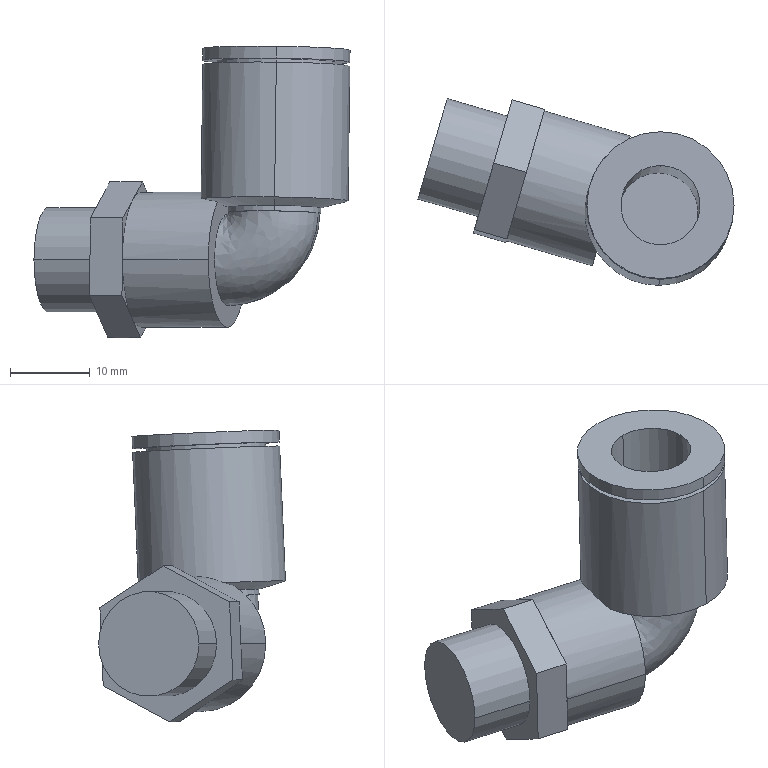Part | SolidWorks | features BaseBody 1 | 1 solid | 38 faces | box 39.742 x 23.493 x 36.691 mm | volume 9283 mm3 | plane 20 | cylinder 14 | cone 2 | spline 2 | commonest cylinder face diameters 18.5 x4 10 x2 11.729 x2 13.157 x2 15 x2 17 x2
STEP:
#1=CARTESIAN_POINT('',(-71.686,422.179,-0.7991));
#2=VERTEX_POINT('',#1);
#3=CARTESIAN_POINT('',(-71.686,403.696,-0.007463));
#4=VERTEX_POINT('',#3);
#5=CARTESIAN_POINT('',(-71.686,412.938,-0.4033));
#6=DIRECTION('',(-0.01248,-0.04279,-0.999));
#7=DIRECTION('',(0.,0.9991,-0.04279));
#8=AXIS2_PLACEMENT_3D('',#5,#6,#7);
#9=CIRCLE('',#8,9.25);
#10=EDGE_CURVE('',#2,#4,#9,.T.);
#11=ORIENTED_EDGE('',*,*,#10,.T.);
#12=CARTESIAN_POINT('',(-71.898,402.97,-16.958));
#13=VERTEX_POINT('',#12);
#14=CARTESIAN_POINT('',(-71.792,403.333,-8.483));
#15=DIRECTION('',(-0.01248,-0.04279,-0.999));
#16=VECTOR('',#15,1000.);
#17=LINE('',#14,#16);
#18=EDGE_CURVE('',#4,#13,#17,.T.);
#19=ORIENTED_EDGE('',*,*,#18,.T.);
#20=CARTESIAN_POINT('',(-71.898,421.453,-17.75));
#21=VERTEX_POINT('',#20);
#22=CARTESIAN_POINT('',(-71.898,412.212,-17.354));
#23=DIRECTION('',(0.01248,0.04279,0.999));
#24=DIRECTION('',(0.,0.9991,-0.04279));
#25=AXIS2_PLACEMENT_3D('',#22,#23,#24);
#26=CIRCLE('',#25,9.25);
#27=EDGE_CURVE('',#13,#21,#26,.T.);
#28=ORIENTED_EDGE('',*,*,#27,.T.);
#29=CARTESIAN_POINT('',(-71.792,421.816,-9.275));
#30=DIRECTION('',(-0.01248,-0.04279,-0.999));
#31=VECTOR('',#30,1000.);
#32=LINE('',#29,#31);
#33=EDGE_CURVE('',#2,#21,#32,.T.);
#34=ORIENTED_EDGE('',*,*,#33,.F.);
#35=EDGE_LOOP('',(#11,#19,#28,#34));
#36=FACE_OUTER_BOUND('',#35,.T.);
#37=CARTESIAN_POINT('',(-71.792,412.575,-8.879));
#38=DIRECTION('',(-0.01248,-0.04279,-0.999));
#39=DIRECTION('',(0.,0.9991,-0.04279));
#40=AXIS2_PLACEMENT_3D('',#37,#38,#39);
#41=CYLINDRICAL_SURFACE('',#40,9.25);
#42=ADVANCED_FACE('',(#36),#41,.T.);
#43=CARTESIAN_POINT('',(-71.909,406.314,-18.01));
#44=VERTEX_POINT('',#43);
#45=CARTESIAN_POINT('',(-71.909,418.032,-18.511));
#46=VERTEX_POINT('',#45);
#47=CARTESIAN_POINT('',(-71.909,412.173,-18.26));
#48=DIRECTION('',(0.01248,0.04279,0.999));
#49=DIRECTION('',(0.2797,0.9591,-0.04457));
#50=AXIS2_PLACEMENT_3D('',#47,#48,#49);
#51=CIRCLE('',#50,5.864);
#52=EDGE_CURVE('',#44,#46,#51,.T.);
#53=ORIENTED_EDGE('',*,*,#52,.T.);
#54=CARTESIAN_POINT('',(-71.898,421.453,-17.75));
#55=DIRECTION('',(0.003229,0.9761,0.2172));
#56=VECTOR('',#55,1000.);
#57=LINE('',#54,#56);
#58=EDGE_CURVE('',#46,#21,#57,.T.);
#59=ORIENTED_EDGE('',*,*,#58,.T.);
#60=ORIENTED_EDGE('',*,*,#27,.F.);
#61=CARTESIAN_POINT('',(-71.898,402.97,-16.958));
#62=DIRECTION('',(0.003229,-0.954,0.2999));
#63=VECTOR('',#62,1000.);
#64=LINE('',#61,#63);
#65=EDGE_CURVE('',#44,#13,#64,.T.);
#66=ORIENTED_EDGE('',*,*,#65,.F.);
#67=EDGE_LOOP('',(#53,#59,#60,#66));
#68=FACE_OUTER_BOUND('',#67,.T.);
#69=CARTESIAN_POINT('',(-71.898,412.212,-17.354));
#70=DIRECTION('',(0.01248,0.04279,0.999));
#71=DIRECTION('',(0.,-0.9991,0.04279));
#72=AXIS2_PLACEMENT_3D('',#69,#70,#71);
#73=CONICAL_SURFACE('',#72,9.25,1.309);
#74=ADVANCED_FACE('',(#68),#73,.T.);
#75=CARTESIAN_POINT('',(-91.031,408.596,-24.5));
#76=VERTEX_POINT('',#75);
#77=CARTESIAN_POINT('',(-91.033,408.588,-24.879));
#78=VERTEX_POINT('',#77);
#79=CARTESIAN_POINT('',(-88.653,416.748,-24.879));
#80=DIRECTION('',(0.96,-0.28,0.));
#81=DIRECTION('',(0.28,0.96,0.));
#82=AXIS2_PLACEMENT_3D('',#79,#80,#81);
#83=CIRCLE('',#82,8.5);
#84=EDGE_CURVE('',#76,#78,#83,.T.);
#85=ORIENTED_EDGE('',*,*,#84,.T.);
#86=CARTESIAN_POINT('',(-80.232,405.438,-24.879));
#87=VERTEX_POINT('',#86);
#88=CARTESIAN_POINT('',(-87.546,407.571,-24.879));
#89=DIRECTION('',(0.96,-0.28,0.));
#90=VECTOR('',#89,1000.);
#91=LINE('',#88,#90);
#92=EDGE_CURVE('',#78,#87,#91,.T.);
#93=ORIENTED_EDGE('',*,*,#92,.T.);
#94=CARTESIAN_POINT('',(-79.066,409.437,-17.567));
#95=VERTEX_POINT('',#94);
#96=CARTESIAN_POINT('',(-77.852,413.598,-24.879));
#97=DIRECTION('',(-0.96,0.28,0.));
#98=DIRECTION('',(0.28,0.96,0.));
#99=AXIS2_PLACEMENT_3D('',#96,#97,#98);
#100=CIRCLE('',#99,8.5);
#101=EDGE_CURVE('',#87,#95,#100,.T.);
#102=ORIENTED_EDGE('',*,*,#101,.T.);
#103=CARTESIAN_POINT('',(-81.034,410.777,-17.179));
#104=VERTEX_POINT('',#103);
#105=CARTESIAN_POINT('',(-81.034,410.777,-17.179));
#106=CARTESIAN_POINT('',(-80.404,410.293,-17.313));
#107=CARTESIAN_POINT('',(-79.746,409.85,-17.445));
#108=CARTESIAN_POINT('',(-79.066,409.437,-17.567));
#109=B_SPLINE_CURVE_WITH_KNOTS('',3,(#105,#106,#107,#108),.UNSPECIFIED.,.F.,.F.,(4,4),(0.,0.002412),.UNSPECIFIED.);
#110=EDGE_CURVE('',#104,#95,#109,.T.);
#111=ORIENTED_EDGE('',*,*,#110,.F.);
#112=CARTESIAN_POINT('',(-78.831,418.333,-17.53));
#113=VERTEX_POINT('',#112);
#114=CARTESIAN_POINT('',(-78.831,418.333,-17.53));
#115=CARTESIAN_POINT('',(-79.25,417.867,-17.202));
#116=CARTESIAN_POINT('',(-79.631,417.344,-16.934));
#117=CARTESIAN_POINT('',(-80.129,416.459,-16.637));
#118=CARTESIAN_POINT('',(-80.281,416.148,-16.558));
#119=CARTESIAN_POINT('',(-80.55,415.511,-16.441));
#120=CARTESIAN_POINT('',(-80.667,415.182,-16.403));
#121=CARTESIAN_POINT('',(-80.964,414.161,-16.356));
#122=CARTESIAN_POINT('',(-81.08,413.476,-16.413));
#123=CARTESIAN_POINT('',(-81.143,412.44,-16.618));
#124=CARTESIAN_POINT('',(-81.145,412.097,-16.707));
#125=CARTESIAN_POINT('',(-81.114,411.427,-16.918));
#126=CARTESIAN_POINT('',(-81.082,411.099,-17.04));
#127=CARTESIAN_POINT('',(-81.034,410.777,-17.179));
#128=B_SPLINE_CURVE_WITH_KNOTS('',3,(#114,#115,#116,#117,#118,#119,#120,#121,#122,#123,#124,#125,#126,#127),.UNSPECIFIED.,.F.,.F.,(4,2,2,2,2,2,4),(-0.004184,-0.002092,-0.001045,0.000001124,0.002094,0.00314,0.004187),.UNSPECIFIED.);
#129=EDGE_CURVE('',#113,#104,#128,.T.);
#130=ORIENTED_EDGE('',*,*,#129,.F.);
#131=CARTESIAN_POINT('',(-76.461,418.369,-17.983));
#132=VERTEX_POINT('',#131);
#133=CARTESIAN_POINT('',(-78.831,418.333,-17.53));
#134=CARTESIAN_POINT('',(-78.043,418.389,-17.69));
#135=CARTESIAN_POINT('',(-77.254,418.397,-17.843));
#136=CARTESIAN_POINT('',(-76.461,418.369,-17.983));
#137=B_SPLINE_CURVE_WITH_KNOTS('',3,(#133,#134,#135,#136),.UNSPECIFIED.,.F.,.F.,(4,4),(0.,0.002412),.UNSPECIFIED.);
#138=EDGE_CURVE('',#113,#132,#137,.T.);
#139=ORIENTED_EDGE('',*,*,#138,.T.);
#140=CARTESIAN_POINT('',(-75.473,421.759,-24.879));
#141=VERTEX_POINT('',#140);
#142=CARTESIAN_POINT('',(-77.852,413.598,-24.879));
#143=DIRECTION('',(-0.96,0.28,0.));
#144=DIRECTION('',(0.28,0.96,0.));
#145=AXIS2_PLACEMENT_3D('',#142,#143,#144);
#146=CIRCLE('',#145,8.5);
#147=EDGE_CURVE('',#132,#141,#146,.T.);
#148=ORIENTED_EDGE('',*,*,#147,.T.);
#149=CARTESIAN_POINT('',(-86.274,424.908,-24.879));
#150=VERTEX_POINT('',#149);
#151=CARTESIAN_POINT('',(-82.787,423.892,-24.879));
#152=DIRECTION('',(0.96,-0.28,0.));
#153=VECTOR('',#152,1000.);
#154=LINE('',#151,#153);
#155=EDGE_CURVE('',#150,#141,#154,.T.);
#156=ORIENTED_EDGE('',*,*,#155,.F.);
#157=CARTESIAN_POINT('',(-87.373,421.139,-17.714));
#158=VERTEX_POINT('',#157);
#159=CARTESIAN_POINT('',(-88.653,416.748,-24.879));
#160=DIRECTION('',(0.96,-0.28,0.));
#161=DIRECTION('',(0.28,0.96,0.));
#162=AXIS2_PLACEMENT_3D('',#159,#160,#161);
#163=CIRCLE('',#162,8.5);
#164=EDGE_CURVE('',#150,#158,#163,.T.);
#165=ORIENTED_EDGE('',*,*,#164,.T.);
#166=CARTESIAN_POINT('',(-89.75,412.987,-17.336));
#167=VERTEX_POINT('',#166);
#168=CARTESIAN_POINT('',(-88.653,416.748,-24.879));
#169=DIRECTION('',(0.96,-0.28,0.));
#170=DIRECTION('',(0.28,0.96,0.));
#171=AXIS2_PLACEMENT_3D('',#168,#169,#170);
#172=CIRCLE('',#171,8.5);
#173=EDGE_CURVE('',#158,#167,#172,.T.);
#174=ORIENTED_EDGE('',*,*,#173,.T.);
#175=CARTESIAN_POINT('',(-88.653,416.748,-24.879));
#176=DIRECTION('',(0.96,-0.28,0.));
#177=DIRECTION('',(0.28,0.96,0.));
#178=AXIS2_PLACEMENT_3D('',#175,#176,#177);
#179=CIRCLE('',#178,8.5);
#180=EDGE_CURVE('',#167,#76,#179,.T.);
#181=ORIENTED_EDGE('',*,*,#180,.T.);
#182=EDGE_LOOP('',(#85,#93,#102,#111,#130,#139,#148,#156,#165,#174,#181));
#183=FACE_OUTER_BOUND('',#182,.T.);
#184=CARTESIAN_POINT('',(-85.167,415.731,-24.879));
#185=DIRECTION('',(0.96,-0.28,0.));
#186=DIRECTION('',(0.28,0.96,0.));
#187=AXIS2_PLACEMENT_3D('',#184,#185,#186);
#188=CYLINDRICAL_SURFACE('',#187,8.5);
#189=ADVANCED_FACE('',(#183),#188,.T.);
#190=CARTESIAN_POINT('',(-71.68,420.452,-0.2247));
#191=VERTEX_POINT('',#190);
#192=CARTESIAN_POINT('',(-71.68,405.466,0.4172));
#193=VERTEX_POINT('',#192);
#194=CARTESIAN_POINT('',(-71.68,412.959,0.09624));
#195=DIRECTION('',(-0.01248,-0.04279,-0.999));
#196=DIRECTION('',(0.,0.9991,-0.04279));
#197=AXIS2_PLACEMENT_3D('',#194,#195,#196);
#198=CIRCLE('',#197,7.5);
#199=EDGE_CURVE('',#191,#193,#198,.T.);
#200=ORIENTED_EDGE('',*,*,#199,.T.);
#201=CARTESIAN_POINT('',(-71.686,405.444,-0.08234));
#202=VERTEX_POINT('',#201);
#203=CARTESIAN_POINT('',(-71.683,405.455,0.1674));
#204=DIRECTION('',(-0.01248,-0.04279,-0.999));
#205=VECTOR('',#204,1000.);
#206=LINE('',#203,#205);
#207=EDGE_CURVE('',#193,#202,#206,.T.);
#208=ORIENTED_EDGE('',*,*,#207,.T.);
#209=CARTESIAN_POINT('',(-71.686,420.431,-0.7242));
#210=VERTEX_POINT('',#209);
#211=CARTESIAN_POINT('',(-71.686,412.938,-0.4033));
#212=DIRECTION('',(-0.01248,-0.04279,-0.999));
#213=DIRECTION('',(0.,0.9991,-0.04279));
#214=AXIS2_PLACEMENT_3D('',#211,#212,#213);
#215=CIRCLE('',#214,7.5);
#216=EDGE_CURVE('',#210,#202,#215,.T.);
#217=ORIENTED_EDGE('',*,*,#216,.F.);
#218=CARTESIAN_POINT('',(-71.683,420.441,-0.4744));
#219=DIRECTION('',(-0.01248,-0.04279,-0.999));
#220=VECTOR('',#219,1000.);
#221=LINE('',#218,#220);
#222=EDGE_CURVE('',#191,#210,#221,.T.);
#223=ORIENTED_EDGE('',*,*,#222,.F.);
#224=EDGE_LOOP('',(#200,#208,#217,#223));
#225=FACE_OUTER_BOUND('',#224,.T.);
#226=CARTESIAN_POINT('',(-71.683,412.948,-0.1535));
#227=DIRECTION('',(-0.01248,-0.04279,-0.999));
#228=DIRECTION('',(0.,0.9991,-0.04279));
#229=AXIS2_PLACEMENT_3D('',#226,#227,#228);
#230=CYLINDRICAL_SURFACE('',#229,7.5);
#231=ADVANCED_FACE('',(#225),#230,.T.);
#232=ORIENTED_EDGE('',*,*,#52,.F.);
#233=CARTESIAN_POINT('',(-71.918,406.284,-18.714));
#234=VERTEX_POINT('',#233);
#235=CARTESIAN_POINT('',(-71.913,406.299,-18.362));
#236=DIRECTION('',(-0.01248,-0.04279,-0.999));
#237=VECTOR('',#236,1000.);
#238=LINE('',#235,#237);
#239=EDGE_CURVE('',#44,#234,#238,.T.);
#240=ORIENTED_EDGE('',*,*,#239,.T.);
#241=CARTESIAN_POINT('',(-71.918,418.002,-19.216));
#242=VERTEX_POINT('',#241);
#243=CARTESIAN_POINT('',(-71.918,412.143,-18.965));
#244=DIRECTION('',(0.01248,0.04279,0.999));
#245=DIRECTION('',(0.,0.9991,-0.04279));
#246=AXIS2_PLACEMENT_3D('',#243,#244,#245);
#247=CIRCLE('',#246,5.864);
#248=EDGE_CURVE('',#234,#242,#247,.T.);
#249=ORIENTED_EDGE('',*,*,#248,.T.);
#250=CARTESIAN_POINT('',(-71.913,418.017,-18.864));
#251=DIRECTION('',(-0.01248,-0.04279,-0.999));
#252=VECTOR('',#251,1000.);
#253=LINE('',#250,#252);
#254=EDGE_CURVE('',#46,#242,#253,.T.);
#255=ORIENTED_EDGE('',*,*,#254,.F.);
#256=EDGE_LOOP('',(#232,#240,#249,#255));
#257=FACE_OUTER_BOUND('',#256,.T.);
#258=CARTESIAN_POINT('',(-71.913,412.158,-18.613));
#259=DIRECTION('',(-0.01248,-0.04279,-0.999));
#260=DIRECTION('',(0.,0.9991,-0.04279));
#261=AXIS2_PLACEMENT_3D('',#258,#259,#260);
#262=CYLINDRICAL_SURFACE('',#261,5.864);
#263=ADVANCED_FACE('',(#257),#262,.T.);
#264=CARTESIAN_POINT('',(-71.661,422.265,1.199));
#265=VERTEX_POINT('',#264);
#266=CARTESIAN_POINT('',(-71.661,403.782,1.991));
#267=VERTEX_POINT('',#266);
#268=CARTESIAN_POINT('',(-71.661,413.023,1.595));
#269=DIRECTION('',(-0.01248,-0.04279,-0.999));
#270=DIRECTION('',(0.,0.9991,-0.04279));
#271=AXIS2_PLACEMENT_3D('',#268,#269,#270);
#272=CIRCLE('',#271,9.25);
#273=EDGE_CURVE('',#265,#267,#272,.T.);
#274=ORIENTED_EDGE('',*,*,#273,.T.);
#275=CARTESIAN_POINT('',(-71.68,403.717,0.492));
#276=VERTEX_POINT('',#275);
#277=CARTESIAN_POINT('',(-71.67,403.75,1.241));
#278=DIRECTION('',(-0.01248,-0.04279,-0.999));
#279=VECTOR('',#278,1000.);
#280=LINE('',#277,#279);
#281=EDGE_CURVE('',#267,#276,#280,.T.);
#282=ORIENTED_EDGE('',*,*,#281,.T.);
#283=CARTESIAN_POINT('',(-71.68,422.201,-0.2996));
#284=VERTEX_POINT('',#283);
#285=CARTESIAN_POINT('',(-71.68,412.959,0.09624));
#286=DIRECTION('',(-0.01248,-0.04279,-0.999));
#287=DIRECTION('',(0.,0.9991,-0.04279));
#288=AXIS2_PLACEMENT_3D('',#285,#286,#287);
#289=CIRCLE('',#288,9.25);
#290=EDGE_CURVE('',#284,#276,#289,.T.);
#291=ORIENTED_EDGE('',*,*,#290,.F.);
#292=CARTESIAN_POINT('',(-71.67,422.233,0.4497));
#293=DIRECTION('',(-0.01248,-0.04279,-0.999));
#294=VECTOR('',#293,1000.);
#295=LINE('',#292,#294);
#296=EDGE_CURVE('',#265,#284,#295,.T.);
#297=ORIENTED_EDGE('',*,*,#296,.F.);
#298=EDGE_LOOP('',(#274,#282,#291,#297));
#299=FACE_OUTER_BOUND('',#298,.T.);
#300=CARTESIAN_POINT('',(-71.67,412.991,0.8455));
#301=DIRECTION('',(-0.01248,-0.04279,-0.999));
#302=DIRECTION('',(0.,0.9991,-0.04279));
#303=AXIS2_PLACEMENT_3D('',#300,#301,#302);
#304=CYLINDRICAL_SURFACE('',#303,9.25);
#305=ADVANCED_FACE('',(#299),#304,.T.);
#306=CARTESIAN_POINT('',(-98.47,426.463,-24.879));
#307=VERTEX_POINT('',#306);
#308=CARTESIAN_POINT('',(-102.154,413.833,-24.879));
#309=VERTEX_POINT('',#308);
#310=CARTESIAN_POINT('',(-100.312,420.148,-24.879));
#311=DIRECTION('',(0.96,-0.28,0.));
#312=DIRECTION('',(0.28,0.96,0.));
#313=AXIS2_PLACEMENT_3D('',#310,#311,#312);
#314=CIRCLE('',#313,6.579);
#315=EDGE_CURVE('',#307,#309,#314,.T.);
#316=ORIENTED_EDGE('',*,*,#315,.T.);
#317=CARTESIAN_POINT('',(-94.575,411.623,-24.879));
#318=VERTEX_POINT('',#317);
#319=CARTESIAN_POINT('',(-98.238,412.691,-24.879));
#320=DIRECTION('',(0.96,-0.28,0.));
#321=VECTOR('',#320,1000.);
#322=LINE('',#319,#321);
#323=EDGE_CURVE('',#309,#318,#322,.T.);
#324=ORIENTED_EDGE('',*,*,#323,.T.);
#325=CARTESIAN_POINT('',(-90.892,424.253,-24.879));
#326=VERTEX_POINT('',#325);
#327=CARTESIAN_POINT('',(-92.733,417.938,-24.879));
#328=DIRECTION('',(-0.96,0.28,0.));
#329=DIRECTION('',(0.28,0.96,0.));
#330=AXIS2_PLACEMENT_3D('',#327,#328,#329);
#331=CIRCLE('',#330,6.579);
#332=EDGE_CURVE('',#318,#326,#331,.T.);
#333=ORIENTED_EDGE('',*,*,#332,.T.);
#334=CARTESIAN_POINT('',(-94.555,425.322,-24.879));
#335=DIRECTION('',(0.96,-0.28,0.));
#336=VECTOR('',#335,1000.);
#337=LINE('',#334,#336);
#338=EDGE_CURVE('',#307,#326,#337,.T.);
#339=ORIENTED_EDGE('',*,*,#338,.F.);
#340=EDGE_LOOP('',(#316,#324,#333,#339));
#341=FACE_OUTER_BOUND('',#340,.T.);
#342=CARTESIAN_POINT('',(-96.396,419.006,-24.879));
#343=DIRECTION('',(0.96,-0.28,0.));
#344=DIRECTION('',(0.28,0.96,0.));
#345=AXIS2_PLACEMENT_3D('',#342,#343,#344);
#346=CYLINDRICAL_SURFACE('',#345,6.579);
#347=ADVANCED_FACE('',(#341),#346,.T.);
#348=CARTESIAN_POINT('',(-71.923,417.12,-19.598));
#349=VERTEX_POINT('',#348);
#350=CARTESIAN_POINT('',(-71.923,407.129,-19.17));
#351=VERTEX_POINT('',#350);
#352=CARTESIAN_POINT('',(-71.923,412.125,-19.384));
#353=DIRECTION('',(0.01248,0.04279,0.999));
#354=DIRECTION('',(0.,-0.9991,0.04279));
#355=AXIS2_PLACEMENT_3D('',#352,#353,#354);
#356=CIRCLE('',#355,5.);
#357=EDGE_CURVE('',#349,#351,#356,.T.);
#358=ORIENTED_EDGE('',*,*,#357,.F.);
#359=CARTESIAN_POINT('',(-71.661,418.019,1.381));
#360=VERTEX_POINT('',#359);
#361=CARTESIAN_POINT('',(-71.399,418.917,22.36));
#362=DIRECTION('',(0.01248,0.04279,0.999));
#363=VECTOR('',#362,1000.);
#364=LINE('',#361,#363);
#365=EDGE_CURVE('',#349,#360,#364,.T.);
#366=ORIENTED_EDGE('',*,*,#365,.T.);
#367=CARTESIAN_POINT('',(-71.661,408.028,1.809));
#368=VERTEX_POINT('',#367);
#369=CARTESIAN_POINT('',(-71.661,413.023,1.595));
#370=DIRECTION('',(-0.01248,-0.04279,-0.999));
#371=DIRECTION('',(0.,-0.9991,0.04279));
#372=AXIS2_PLACEMENT_3D('',#369,#370,#371);
#373=CIRCLE('',#372,5.);
#374=EDGE_CURVE('',#368,#360,#373,.T.);
#375=ORIENTED_EDGE('',*,*,#374,.F.);
#376=CARTESIAN_POINT('',(-71.399,408.926,22.788));
#377=DIRECTION('',(0.01248,0.04279,0.999));
#378=VECTOR('',#377,1000.);
#379=LINE('',#376,#378);
#380=EDGE_CURVE('',#351,#368,#379,.T.);
#381=ORIENTED_EDGE('',*,*,#380,.F.);
#382=EDGE_LOOP('',(#358,#366,#375,#381));
#383=FACE_OUTER_BOUND('',#382,.T.);
#384=CARTESIAN_POINT('',(-71.399,413.922,22.574));
#385=DIRECTION('',(0.01248,0.04279,0.999));
#386=DIRECTION('',(0.,-0.9991,0.04279));
#387=AXIS2_PLACEMENT_3D('',#384,#385,#386);
#388=CYLINDRICAL_SURFACE('',#387,5.);
#389=ADVANCED_FACE('',(#383),#388,.F.);
#390=ORIENTED_EDGE('',*,*,#18,.F.);
#391=CARTESIAN_POINT('',(-71.686,412.938,-0.4033));
#392=DIRECTION('',(-0.01248,-0.04279,-0.999));
#393=DIRECTION('',(0.,0.9991,-0.04279));
#394=AXIS2_PLACEMENT_3D('',#391,#392,#393);
#395=CIRCLE('',#394,9.25);
#396=EDGE_CURVE('',#4,#2,#395,.T.);
#397=ORIENTED_EDGE('',*,*,#396,.T.);
#398=ORIENTED_EDGE('',*,*,#33,.T.);
#399=CARTESIAN_POINT('',(-71.898,412.212,-17.354));
#400=DIRECTION('',(0.01248,0.04279,0.999));
#401=DIRECTION('',(0.,0.9991,-0.04279));
#402=AXIS2_PLACEMENT_3D('',#399,#400,#401);
#403=CIRCLE('',#402,9.25);
#404=EDGE_CURVE('',#21,#113,#403,.T.);
#405=ORIENTED_EDGE('',*,*,#404,.T.);
#406=ORIENTED_EDGE('',*,*,#129,.T.);
#407=CARTESIAN_POINT('',(-71.898,412.212,-17.354));
#408=DIRECTION('',(0.01248,0.04279,0.999));
#409=DIRECTION('',(0.,0.9991,-0.04279));
#410=AXIS2_PLACEMENT_3D('',#407,#408,#409);
#411=CIRCLE('',#410,9.25);
#412=EDGE_CURVE('',#104,#13,#411,.T.);
#413=ORIENTED_EDGE('',*,*,#412,.T.);
#414=EDGE_LOOP('',(#390,#397,#398,#405,#406,#413));
#415=FACE_OUTER_BOUND('',#414,.T.);
#416=CARTESIAN_POINT('',(-71.792,412.575,-8.879));
#417=DIRECTION('',(-0.01248,-0.04279,-0.999));
#418=DIRECTION('',(0.,0.9991,-0.04279));
#419=AXIS2_PLACEMENT_3D('',#416,#417,#418);
#420=CYLINDRICAL_SURFACE('',#419,9.25);
#421=ADVANCED_FACE('',(#415),#420,.T.);
#422=ORIENTED_EDGE('',*,*,#216,.T.);
#423=CARTESIAN_POINT('',(-71.686,412.938,-0.4033));
#424=DIRECTION('',(-0.01248,-0.04279,-0.999));
#425=DIRECTION('',(0.,0.9991,-0.04279));
#426=AXIS2_PLACEMENT_3D('',#423,#424,#425);
#427=CIRCLE('',#426,7.5);
#428=EDGE_CURVE('',#202,#210,#427,.T.);
#429=ORIENTED_EDGE('',*,*,#428,.T.);
#430=EDGE_LOOP('',(#422,#429));
#431=FACE_BOUND('',#430,.T.);
#432=ORIENTED_EDGE('',*,*,#10,.F.);
#433=ORIENTED_EDGE('',*,*,#396,.F.);
#434=EDGE_LOOP('',(#432,#433));
#435=FACE_OUTER_BOUND('',#434,.T.);
#436=CARTESIAN_POINT('',(-69.344,420.97,-0.7765));
#437=DIRECTION('',(0.01248,0.04279,0.999));
#438=DIRECTION('',(0.,-0.9991,0.04279));
#439=AXIS2_PLACEMENT_3D('',#436,#437,#438);
#440=PLANE('',#439);
#441=ADVANCED_FACE('',(#431,#435),#440,.T.);
#442=ORIENTED_EDGE('',*,*,#58,.F.);
#443=CARTESIAN_POINT('',(-71.909,412.173,-18.26));
#444=DIRECTION('',(0.01248,0.04279,0.999));
#445=DIRECTION('',(0.2797,0.9591,-0.04457));
#446=AXIS2_PLACEMENT_3D('',#443,#444,#445);
#447=CIRCLE('',#446,5.864);
#448=EDGE_CURVE('',#46,#44,#447,.T.);
#449=ORIENTED_EDGE('',*,*,#448,.T.);
#450=ORIENTED_EDGE('',*,*,#65,.T.);
#451=ORIENTED_EDGE('',*,*,#412,.F.);
#452=ORIENTED_EDGE('',*,*,#110,.T.);
#453=CARTESIAN_POINT('',(-79.066,409.437,-17.567));
#454=CARTESIAN_POINT('',(-78.852,410.171,-17.727));
#455=CARTESIAN_POINT('',(-78.637,410.908,-17.868));
#456=CARTESIAN_POINT('',(-78.205,412.389,-18.085));
#457=CARTESIAN_POINT('',(-77.988,413.134,-18.161));
#458=CARTESIAN_POINT('',(-77.55,414.635,-18.231));
#459=CARTESIAN_POINT('',(-77.332,415.384,-18.224));
#460=CARTESIAN_POINT('',(-76.896,416.878,-18.145));
#461=CARTESIAN_POINT('',(-76.679,417.624,-18.073));
#462=CARTESIAN_POINT('',(-76.461,418.369,-17.983));
#463=B_SPLINE_CURVE_WITH_KNOTS('',3,(#453,#454,#455,#456,#457,#458,#459,#460,#461,#462),.UNSPECIFIED.,.F.,.F.,(4,2,2,2,4),(0.,0.002338,0.004676,0.007013,0.009351),.UNSPECIFIED.);
#464=EDGE_CURVE('',#95,#132,#463,.T.);
#465=ORIENTED_EDGE('',*,*,#464,.T.);
#466=ORIENTED_EDGE('',*,*,#138,.F.);
#467=ORIENTED_EDGE('',*,*,#404,.F.);
#468=EDGE_LOOP('',(#442,#449,#450,#451,#452,#465,#466,#467));
#469=FACE_OUTER_BOUND('',#468,.T.);
#470=CARTESIAN_POINT('',(-71.898,412.212,-17.354));
#471=DIRECTION('',(0.01248,0.04279,0.999));
#472=DIRECTION('',(0.,-0.9991,0.04279));
#473=AXIS2_PLACEMENT_3D('',#470,#471,#472);
#474=CONICAL_SURFACE('',#473,9.25,1.309);
#475=ADVANCED_FACE('',(#469),#474,.T.);
#476=ORIENTED_EDGE('',*,*,#92,.F.);
#477=CARTESIAN_POINT('',(-89.934,412.357,-32.043));
#478=VERTEX_POINT('',#477);
#479=CARTESIAN_POINT('',(-88.653,416.748,-24.879));
#480=DIRECTION('',(0.96,-0.28,0.));
#481=DIRECTION('',(0.28,0.96,0.));
#482=AXIS2_PLACEMENT_3D('',#479,#480,#481);
#483=CIRCLE('',#482,8.5);
#484=EDGE_CURVE('',#78,#478,#483,.T.);
#485=ORIENTED_EDGE('',*,*,#484,.T.);
#486=CARTESIAN_POINT('',(-87.557,420.509,-32.422));
#487=VERTEX_POINT('',#486);
#488=CARTESIAN_POINT('',(-88.653,416.748,-24.879));
#489=DIRECTION('',(0.96,-0.28,0.));
#490=DIRECTION('',(0.28,0.96,0.));
#491=AXIS2_PLACEMENT_3D('',#488,#489,#490);
#492=CIRCLE('',#491,8.5);
#493=EDGE_CURVE('',#478,#487,#492,.T.);
#494=ORIENTED_EDGE('',*,*,#493,.T.);
#495=CARTESIAN_POINT('',(-86.276,424.9,-25.258));
#496=VERTEX_POINT('',#495);
#497=CARTESIAN_POINT('',(-88.653,416.748,-24.879));
#498=DIRECTION('',(0.96,-0.28,0.));
#499=DIRECTION('',(0.28,0.96,0.));
#500=AXIS2_PLACEMENT_3D('',#497,#498,#499);
#501=CIRCLE('',#500,8.5);
#502=EDGE_CURVE('',#487,#496,#501,.T.);
#503=ORIENTED_EDGE('',*,*,#502,.T.);
#504=CARTESIAN_POINT('',(-88.653,416.748,-24.879));
#505=DIRECTION('',(0.96,-0.28,0.));
#506=DIRECTION('',(0.28,0.96,0.));
#507=AXIS2_PLACEMENT_3D('',#504,#505,#506);
#508=CIRCLE('',#507,8.5);
#509=EDGE_CURVE('',#496,#150,#508,.T.);
#510=ORIENTED_EDGE('',*,*,#509,.T.);
#511=ORIENTED_EDGE('',*,*,#155,.T.);
#512=CARTESIAN_POINT('',(-77.852,413.598,-24.879));
#513=DIRECTION('',(-0.96,0.28,0.));
#514=DIRECTION('',(0.28,0.96,0.));
#515=AXIS2_PLACEMENT_3D('',#512,#513,#514);
#516=CIRCLE('',#515,8.5);
#517=EDGE_CURVE('',#141,#87,#516,.T.);
#518=ORIENTED_EDGE('',*,*,#517,.T.);
#519=EDGE_LOOP('',(#476,#485,#494,#503,#510,#511,#518));
#520=FACE_OUTER_BOUND('',#519,.T.);
#521=CARTESIAN_POINT('',(-85.167,415.731,-24.879));
#522=DIRECTION('',(0.96,-0.28,0.));
#523=DIRECTION('',(0.28,0.96,0.));
#524=AXIS2_PLACEMENT_3D('',#521,#522,#523);
#525=CYLINDRICAL_SURFACE('',#524,8.5);
#526=ADVANCED_FACE('',(#520),#525,.T.);
#527=ORIENTED_EDGE('',*,*,#207,.F.);
#528=CARTESIAN_POINT('',(-71.68,412.959,0.09624));
#529=DIRECTION('',(-0.01248,-0.04279,-0.999));
#530=DIRECTION('',(0.,0.9991,-0.04279));
#531=AXIS2_PLACEMENT_3D('',#528,#529,#530);
#532=CIRCLE('',#531,7.5);
#533=EDGE_CURVE('',#193,#191,#532,.T.);
#534=ORIENTED_EDGE('',*,*,#533,.T.);
#535=ORIENTED_EDGE('',*,*,#222,.T.);
#536=ORIENTED_EDGE('',*,*,#428,.F.);
#537=EDGE_LOOP('',(#527,#534,#535,#536));
#538=FACE_OUTER_BOUND('',#537,.T.);
#539=CARTESIAN_POINT('',(-71.683,412.948,-0.1535));
#540=DIRECTION('',(-0.01248,-0.04279,-0.999));
#541=DIRECTION('',(0.,0.9991,-0.04279));
#542=AXIS2_PLACEMENT_3D('',#539,#540,#541);
#543=CYLINDRICAL_SURFACE('',#542,7.5);
#544=ADVANCED_FACE('',(#538),#543,.T.);
#545=ORIENTED_EDGE('',*,*,#464,.F.);
#546=ORIENTED_EDGE('',*,*,#101,.F.);
#547=ORIENTED_EDGE('',*,*,#517,.F.);
#548=ORIENTED_EDGE('',*,*,#147,.F.);
#549=EDGE_LOOP('',(#545,#546,#547,#548));
#550=FACE_OUTER_BOUND('',#549,.T.);
#551=CARTESIAN_POINT('',(-77.924,413.353,-30.608));
#552=VERTEX_POINT('',#551);
#553=CARTESIAN_POINT('',(-77.781,413.844,-19.15));
#554=VERTEX_POINT('',#553);
#555=CARTESIAN_POINT('',(-77.924,413.353,-30.608));
#556=CARTESIAN_POINT('',(-78.03,412.99,-30.591));
#557=CARTESIAN_POINT('',(-78.134,412.634,-30.538));
#558=CARTESIAN_POINT('',(-78.286,412.112,-30.404));
#559=CARTESIAN_POINT('',(-78.336,411.939,-30.351));
#560=CARTESIAN_POINT('',(-78.436,411.598,-30.225));
#561=CARTESIAN_POINT('',(-78.485,411.429,-30.153));
#562=CARTESIAN_POINT('',(-78.628,410.939,-29.915));
#563=CARTESIAN_POINT('',(-78.718,410.631,-29.724));
#564=CARTESIAN_POINT('',(-78.887,410.051,-29.281));
#565=CARTESIAN_POINT('',(-78.967,409.778,-29.025));
#566=CARTESIAN_POINT('',(-79.108,409.293,-28.473));
#567=CARTESIAN_POINT('',(-79.171,409.078,-28.174));
#568=CARTESIAN_POINT('',(-79.253,408.797,-27.691));
#569=CARTESIAN_POINT('',(-79.278,408.71,-27.524));
#570=CARTESIAN_POINT('',(-79.323,408.554,-27.185));
#571=CARTESIAN_POINT('',(-79.344,408.485,-27.013));
#572=CARTESIAN_POINT('',(-79.397,408.301,-26.486));
#573=CARTESIAN_POINT('',(-79.423,408.211,-26.12));
#574=CARTESIAN_POINT('',(-79.455,408.101,-25.374));
#575=CARTESIAN_POINT('',(-79.461,408.082,-25.001));
#576=CARTESIAN_POINT('',(-79.452,408.114,-24.254));
#577=CARTESIAN_POINT('',(-79.437,408.166,-23.876));
#578=CARTESIAN_POINT('',(-79.387,408.337,-23.148));
#579=CARTESIAN_POINT('',(-79.352,408.456,-22.795));
#580=CARTESIAN_POINT('',(-79.285,408.685,-22.285));
#581=CARTESIAN_POINT('',(-79.26,408.77,-22.116));
#582=CARTESIAN_POINT('',(-79.207,408.955,-21.792));
#583=CARTESIAN_POINT('',(-79.178,409.054,-21.636));
#584=CARTESIAN_POINT('',(-79.085,409.372,-21.184));
#585=CARTESIAN_POINT('',(-79.015,409.612,-20.905));
#586=CARTESIAN_POINT('',(-78.859,410.148,-20.394));
#587=CARTESIAN_POINT('',(-78.775,410.436,-20.169));
#588=CARTESIAN_POINT('',(-78.64,410.896,-19.879));
#589=CARTESIAN_POINT('',(-78.594,411.054,-19.79));
#590=CARTESIAN_POINT('',(-78.499,411.38,-19.627));
#591=CARTESIAN_POINT('',(-78.45,411.548,-19.553));
#592=CARTESIAN_POINT('',(-78.302,412.057,-19.36));
#593=CARTESIAN_POINT('',(-78.201,412.405,-19.268));
#594=CARTESIAN_POINT('',(-77.993,413.115,-19.154));
#595=CARTESIAN_POINT('',(-77.887,413.481,-19.133));
#596=CARTESIAN_POINT('',(-77.781,413.844,-19.15));
#597=B_SPLINE_CURVE_WITH_KNOTS('',3,(#555,#556,#557,#558,#559,#560,#561,#562,#563,#564,#565,#566,#567,#568,#569,#570,#571,#572,#573,#574,#575,#576,#577,#578,#579,#580,#581,#582,#583,#584,#585,#586,#587,#588,#589,#590,#591,#592,#593,#594,#595,#596),.UNSPECIFIED.,.F.,.F.,(4,2,2,2,2,2,2,2,2,2,2,2,2,2,2,2,2,2,2,2,4),(0.,0.00112,0.001681,0.002241,0.003361,0.004482,0.005602,0.006162,0.006722,0.007843,0.008963,0.01008,0.0112,0.01176,0.01232,0.01344,0.01457,0.01513,0.01569,0.01681,0.01793),.UNSPECIFIED.);
#598=EDGE_CURVE('',#552,#554,#597,.T.);
#599=ORIENTED_EDGE('',*,*,#598,.T.);
#600=CARTESIAN_POINT('',(-77.781,413.844,-19.15));
#601=CARTESIAN_POINT('',(-77.675,414.207,-19.166));
#602=CARTESIAN_POINT('',(-77.569,414.569,-19.221));
#603=CARTESIAN_POINT('',(-77.365,415.269,-19.401));
#604=CARTESIAN_POINT('',(-77.267,415.607,-19.526));
#605=CARTESIAN_POINT('',(-77.077,416.259,-19.844));
#606=CARTESIAN_POINT('',(-76.985,416.574,-20.039));
#607=CARTESIAN_POINT('',(-76.816,417.152,-20.482));
#608=CARTESIAN_POINT('',(-76.738,417.419,-20.732));
#609=CARTESIAN_POINT('',(-76.596,417.908,-21.29));
#610=CARTESIAN_POINT('',(-76.533,418.124,-21.592));
#611=CARTESIAN_POINT('',(-76.452,418.402,-22.071));
#612=CARTESIAN_POINT('',(-76.427,418.488,-22.235));
#613=CARTESIAN_POINT('',(-76.381,418.643,-22.574));
#614=CARTESIAN_POINT('',(-76.361,418.714,-22.749));
#615=CARTESIAN_POINT('',(-76.307,418.898,-23.281));
#616=CARTESIAN_POINT('',(-76.281,418.987,-23.643));
#617=CARTESIAN_POINT('',(-76.249,419.095,-24.383));
#618=CARTESIAN_POINT('',(-76.244,419.115,-24.764));
#619=CARTESIAN_POINT('',(-76.253,419.082,-25.512));
#620=CARTESIAN_POINT('',(-76.268,419.031,-25.882));
#621=CARTESIAN_POINT('',(-76.306,418.902,-26.43));
#622=CARTESIAN_POINT('',(-76.321,418.85,-26.612));
#623=CARTESIAN_POINT('',(-76.356,418.73,-26.966));
#624=CARTESIAN_POINT('',(-76.376,418.662,-27.14));
#625=CARTESIAN_POINT('',(-76.442,418.434,-27.647));
#626=CARTESIAN_POINT('',(-76.496,418.25,-27.97));
#627=CARTESIAN_POINT('',(-76.621,417.82,-28.58));
#628=CARTESIAN_POINT('',(-76.691,417.58,-28.858));
#629=CARTESIAN_POINT('',(-76.807,417.183,-29.236));
#630=CARTESIAN_POINT('',(-76.848,417.044,-29.356));
#631=CARTESIAN_POINT('',(-76.932,416.755,-29.582));
#632=CARTESIAN_POINT('',(-76.976,416.604,-29.688));
#633=CARTESIAN_POINT('',(-77.111,416.141,-29.98));
#634=CARTESIAN_POINT('',(-77.205,415.818,-30.141));
#635=CARTESIAN_POINT('',(-77.403,415.141,-30.397));
#636=CARTESIAN_POINT('',(-77.506,414.786,-30.491));
#637=CARTESIAN_POINT('',(-77.713,414.076,-30.605));
#638=CARTESIAN_POINT('',(-77.818,413.716,-30.625));
#639=CARTESIAN_POINT('',(-77.924,413.353,-30.608));
#640=B_SPLINE_CURVE_WITH_KNOTS('',3,(#600,#601,#602,#603,#604,#605,#606,#607,#608,#609,#610,#611,#612,#613,#614,#615,#616,#617,#618,#619,#620,#621,#622,#623,#624,#625,#626,#627,#628,#629,#630,#631,#632,#633,#634,#635,#636,#637,#638,#639),.UNSPECIFIED.,.F.,.F.,(4,2,2,2,2,2,2,2,2,2,2,2,2,2,2,2,2,2,2,4),(0.,0.001134,0.002268,0.003402,0.004536,0.00567,0.006237,0.006804,0.007938,0.009072,0.01021,0.01077,0.01134,0.01247,0.01361,0.01417,0.01474,0.01588,0.01701,0.01814),.UNSPECIFIED.);
#641=EDGE_CURVE('',#554,#552,#640,.T.);
#642=ORIENTED_EDGE('',*,*,#641,.T.);
#643=EDGE_LOOP('',(#599,#642));
#644=FACE_BOUND('',#643,.T.);
#645=CARTESIAN_POINT('',(-76.664,417.674,-25.068));
#646=DIRECTION('',(0.96,-0.28,0.));
#647=DIRECTION('',(0.28,0.96,0.));
#648=AXIS2_PLACEMENT_3D('',#645,#646,#647);
#649=PLANE('',#648);
#650=ADVANCED_FACE('',(#550,#644),#649,.T.);
#651=ORIENTED_EDGE('',*,*,#239,.F.);
#652=ORIENTED_EDGE('',*,*,#448,.F.);
#653=ORIENTED_EDGE('',*,*,#254,.T.);
#654=CARTESIAN_POINT('',(-71.918,412.143,-18.965));
#655=DIRECTION('',(0.01248,0.04279,0.999));
#656=DIRECTION('',(0.,0.9991,-0.04279));
#657=AXIS2_PLACEMENT_3D('',#654,#655,#656);
#658=CIRCLE('',#657,5.864);
#659=EDGE_CURVE('',#242,#234,#658,.T.);
#660=ORIENTED_EDGE('',*,*,#659,.T.);
#661=EDGE_LOOP('',(#651,#652,#653,#660));
#662=FACE_OUTER_BOUND('',#661,.T.);
#663=CARTESIAN_POINT('',(-71.913,412.158,-18.613));
#664=DIRECTION('',(-0.01248,-0.04279,-0.999));
#665=DIRECTION('',(0.,0.9991,-0.04279));
#666=AXIS2_PLACEMENT_3D('',#663,#664,#665);
#667=CYLINDRICAL_SURFACE('',#666,5.864);
#668=ADVANCED_FACE('',(#662),#667,.T.);
#669=CARTESIAN_POINT('',(-90.969,408.806,-19.597));
#670=VERTEX_POINT('',#669);
#671=CARTESIAN_POINT('',(-90.969,408.806,-19.597));
#672=DIRECTION('',(-0.01248,-0.04279,-0.999));
#673=VECTOR('',#672,1000.);
#674=LINE('',#671,#673);
#675=EDGE_CURVE('',#670,#76,#674,.T.);
#676=ORIENTED_EDGE('',*,*,#675,.T.);
#677=ORIENTED_EDGE('',*,*,#180,.F.);
#678=CARTESIAN_POINT('',(-89.75,412.987,-17.336));
#679=DIRECTION('',(-0.2484,-0.852,-0.4609));
#680=VECTOR('',#679,1000.);
#681=LINE('',#678,#680);
#682=EDGE_CURVE('',#167,#670,#681,.T.);
#683=ORIENTED_EDGE('',*,*,#682,.T.);
#684=EDGE_LOOP('',(#676,#677,#683));
#685=FACE_OUTER_BOUND('',#684,.T.);
#686=CARTESIAN_POINT('',(-88.653,416.748,-24.879));
#687=DIRECTION('',(0.96,-0.28,0.));
#688=DIRECTION('',(0.28,0.96,0.));
#689=AXIS2_PLACEMENT_3D('',#686,#687,#688);
#690=PLANE('',#689);
#691=ADVANCED_FACE('',(#685),#690,.T.);
#692=CARTESIAN_POINT('',(-88.531,417.168,-15.074));
#693=VERTEX_POINT('',#692);
#694=CARTESIAN_POINT('',(-88.531,417.168,-15.074));
#695=DIRECTION('',(-0.2484,-0.852,-0.4609));
#696=VECTOR('',#695,1000.);
#697=LINE('',#694,#696);
#698=EDGE_CURVE('',#693,#167,#697,.T.);
#699=ORIENTED_EDGE('',*,*,#698,.T.);
#700=ORIENTED_EDGE('',*,*,#173,.F.);
#701=CARTESIAN_POINT('',(-87.373,421.139,-17.714));
#702=DIRECTION('',(-0.236,-0.8092,0.5381));
#703=VECTOR('',#702,1000.);
#704=LINE('',#701,#703);
#705=EDGE_CURVE('',#158,#693,#704,.T.);
#706=ORIENTED_EDGE('',*,*,#705,.T.);
#707=EDGE_LOOP('',(#699,#700,#706));
#708=FACE_OUTER_BOUND('',#707,.T.);
#709=CARTESIAN_POINT('',(-88.653,416.748,-24.879));
#710=DIRECTION('',(0.96,-0.28,0.));
#711=DIRECTION('',(0.28,0.96,0.));
#712=AXIS2_PLACEMENT_3D('',#709,#710,#711);
#713=PLANE('',#712);
#714=ADVANCED_FACE('',(#708),#713,.T.);
#715=CARTESIAN_POINT('',(-86.215,425.11,-20.355));
#716=VERTEX_POINT('',#715);
#717=CARTESIAN_POINT('',(-86.215,425.11,-20.355));
#718=DIRECTION('',(-0.236,-0.8092,0.5381));
#719=VECTOR('',#718,1000.);
#720=LINE('',#717,#719);
#721=EDGE_CURVE('',#716,#158,#720,.T.);
#722=ORIENTED_EDGE('',*,*,#721,.T.);
#723=ORIENTED_EDGE('',*,*,#164,.F.);
#724=ORIENTED_EDGE('',*,*,#509,.F.);
#725=CARTESIAN_POINT('',(-86.276,424.9,-25.258));
#726=DIRECTION('',(0.01248,0.04279,0.999));
#727=VECTOR('',#726,1000.);
#728=LINE('',#725,#727);
#729=EDGE_CURVE('',#496,#716,#728,.T.);
#730=ORIENTED_EDGE('',*,*,#729,.T.);
#731=EDGE_LOOP('',(#722,#723,#724,#730));
#732=FACE_OUTER_BOUND('',#731,.T.);
#733=CARTESIAN_POINT('',(-88.653,416.748,-24.879));
#734=DIRECTION('',(0.96,-0.28,0.));
#735=DIRECTION('',(0.28,0.96,0.));
#736=AXIS2_PLACEMENT_3D('',#733,#734,#735);
#737=PLANE('',#736);
#738=ADVANCED_FACE('',(#732),#737,.T.);
#739=ORIENTED_EDGE('',*,*,#290,.T.);
#740=CARTESIAN_POINT('',(-71.68,412.959,0.09624));
#741=DIRECTION('',(-0.01248,-0.04279,-0.999));
#742=DIRECTION('',(0.,0.9991,-0.04279));
#743=AXIS2_PLACEMENT_3D('',#740,#741,#742);
#744=CIRCLE('',#743,9.25);
#745=EDGE_CURVE('',#276,#284,#744,.T.);
#746=ORIENTED_EDGE('',*,*,#745,.T.);
#747=EDGE_LOOP('',(#739,#746));
#748=FACE_OUTER_BOUND('',#747,.T.);
#749=ORIENTED_EDGE('',*,*,#199,.F.);
#750=ORIENTED_EDGE('',*,*,#533,.F.);
#751=EDGE_LOOP('',(#749,#750));
#752=FACE_BOUND('',#751,.T.);
#753=CARTESIAN_POINT('',(-69.337,420.991,-0.277));
#754=DIRECTION('',(-0.01248,-0.04279,-0.999));
#755=DIRECTION('',(0.,0.9991,-0.04279));
#756=AXIS2_PLACEMENT_3D('',#753,#754,#755);
#757=PLANE('',#756);
#758=ADVANCED_FACE('',(#748,#752),#757,.T.);
#759=CARTESIAN_POINT('',(-66.413,410.538,-18.965));
#760=VERTEX_POINT('',#759);
#761=CARTESIAN_POINT('',(-66.413,410.538,-18.965));
#762=CARTESIAN_POINT('',(-66.602,410.274,-25.813));
#763=CARTESIAN_POINT('',(-71.353,411.437,-30.608));
#764=CARTESIAN_POINT('',(-77.924,413.353,-30.608));
#765=(BOUNDED_CURVE()B_SPLINE_CURVE(3,(#761,#762,#763,#764),.UNSPECIFIED.,.F.,.F.)B_SPLINE_CURVE_WITH_KNOTS((4,4),(0.006606,1.),.UNSPECIFIED.)CURVE()GEOMETRIC_REPRESENTATION_ITEM()RATIONAL_B_SPLINE_CURVE((0.9962,0.8062,0.8075,1.))REPRESENTATION_ITEM(''));
#766=EDGE_CURVE('',#760,#552,#765,.T.);
#767=ORIENTED_EDGE('',*,*,#766,.T.);
#768=ORIENTED_EDGE('',*,*,#641,.F.);
#769=CARTESIAN_POINT('',(-77.471,413.762,-18.965));
#770=VERTEX_POINT('',#769);
#771=CARTESIAN_POINT('',(-77.781,413.844,-19.15));
#772=CARTESIAN_POINT('',(-77.654,413.807,-19.15));
#773=CARTESIAN_POINT('',(-77.539,413.776,-19.085));
#774=CARTESIAN_POINT('',(-77.471,413.762,-18.965));
#775=(BOUNDED_CURVE()B_SPLINE_CURVE(3,(#771,#772,#773,#774),.UNSPECIFIED.,.F.,.T.)B_SPLINE_CURVE_WITH_KNOTS((4,4),(0.001639,0.6632),.UNSPECIFIED.)CURVE()GEOMETRIC_REPRESENTATION_ITEM()RATIONAL_B_SPLINE_CURVE((1.,0.8718,0.8284,0.8698))REPRESENTATION_ITEM(''));
#776=EDGE_CURVE('',#554,#770,#775,.T.);
#777=ORIENTED_EDGE('',*,*,#776,.T.);
#778=CARTESIAN_POINT('',(-77.471,413.762,-18.965));
#779=CARTESIAN_POINT('',(-77.365,414.126,-18.982));
#780=CARTESIAN_POINT('',(-77.216,414.477,-18.999));
#781=CARTESIAN_POINT('',(-76.858,415.137,-19.031));
#782=CARTESIAN_POINT('',(-76.649,415.446,-19.047));
#783=CARTESIAN_POINT('',(-76.174,416.026,-19.078));
#784=CARTESIAN_POINT('',(-75.905,416.297,-19.093));
#785=CARTESIAN_POINT('',(-75.33,416.775,-19.121));
#786=CARTESIAN_POINT('',(-75.021,416.986,-19.133));
#787=CARTESIAN_POINT('',(-74.525,417.257,-19.151));
#788=CARTESIAN_POINT('',(-74.354,417.34,-19.157));
#789=CARTESIAN_POINT('',(-74.008,417.487,-19.168));
#790=CARTESIAN_POINT('',(-73.833,417.552,-19.173));
#791=CARTESIAN_POINT('',(-73.298,417.72,-19.186));
#792=CARTESIAN_POINT('',(-72.93,417.798,-19.194));
#793=CARTESIAN_POINT('',(-72.178,417.88,-19.207));
#794=CARTESIAN_POINT('',(-71.804,417.884,-19.212));
#795=CARTESIAN_POINT('',(-71.245,417.836,-19.217));
#796=CARTESIAN_POINT('',(-71.059,417.811,-19.218));
#797=CARTESIAN_POINT('',(-70.688,417.742,-19.22));
#798=CARTESIAN_POINT('',(-70.503,417.698,-19.22));
#799=CARTESIAN_POINT('',(-69.962,417.541,-19.22));
#800=CARTESIAN_POINT('',(-69.615,417.402,-19.219));
#801=CARTESIAN_POINT('',(-68.948,417.056,-19.212));
#802=CARTESIAN_POINT('',(-68.628,416.848,-19.207));
#803=CARTESIAN_POINT('',(-68.044,416.381,-19.195));
#804=CARTESIAN_POINT('',(-67.776,416.12,-19.187));
#805=CARTESIAN_POINT('',(-67.289,415.541,-19.168));
#806=CARTESIAN_POINT('',(-67.076,415.23,-19.158));
#807=CARTESIAN_POINT('',(-66.805,414.739,-19.14));
#808=CARTESIAN_POINT('',(-66.723,414.571,-19.134));
#809=CARTESIAN_POINT('',(-66.575,414.226,-19.121));
#810=CARTESIAN_POINT('',(-66.509,414.048,-19.114));
#811=CARTESIAN_POINT('',(-66.338,413.509,-19.093));
#812=CARTESIAN_POINT('',(-66.261,413.143,-19.078));
#813=CARTESIAN_POINT('',(-66.178,412.399,-19.047));
#814=CARTESIAN_POINT('',(-66.174,412.018,-19.031));
#815=CARTESIAN_POINT('',(-66.239,411.27,-18.998));
#816=CARTESIAN_POINT('',(-66.307,410.901,-18.982));
#817=CARTESIAN_POINT('',(-66.413,410.538,-18.965));
#818=B_SPLINE_CURVE_WITH_KNOTS('',3,(#778,#779,#780,#781,#782,#783,#784,#785,#786,#787,#788,#789,#790,#791,#792,#793,#794,#795,#796,#797,#798,#799,#800,#801,#802,#803,#804,#805,#806,#807,#808,#809,#810,#811,#812,#813,#814,#815,#816,#817),.UNSPECIFIED.,.F.,.F.,(4,2,2,2,2,2,2,2,2,2,2,2,2,2,2,2,2,2,2,4),(0.,0.001135,0.00227,0.003405,0.00454,0.005107,0.005675,0.00681,0.007945,0.008512,0.00908,0.01021,0.01135,0.01248,0.01362,0.01419,0.01475,0.01589,0.01702,0.01816),.UNSPECIFIED.);
#819=EDGE_CURVE('',#770,#760,#818,.T.);
#820=ORIENTED_EDGE('',*,*,#819,.T.);
#821=EDGE_LOOP('',(#767,#768,#777,#820));
#822=FACE_OUTER_BOUND('',#821,.T.);
#823=CARTESIAN_POINT('',(-77.421,413.756,-18.783));
#824=CARTESIAN_POINT('',(-77.426,413.747,-18.998));
#825=CARTESIAN_POINT('',(-77.574,413.784,-19.15));
#826=CARTESIAN_POINT('',(-77.781,413.844,-19.15));
#827=CARTESIAN_POINT('',(-74.213,424.756,-19.294));
#828=CARTESIAN_POINT('',(-74.218,424.748,-19.509));
#829=CARTESIAN_POINT('',(-74.366,424.784,-19.661));
#830=CARTESIAN_POINT('',(-74.573,424.844,-19.661));
#831=CARTESIAN_POINT('',(-63.204,421.541,-19.393));
#832=CARTESIAN_POINT('',(-63.346,421.263,-26.276));
#833=CARTESIAN_POINT('',(-68.104,422.425,-31.119));
#834=CARTESIAN_POINT('',(-74.716,424.354,-31.119));
#835=CARTESIAN_POINT('',(-66.411,410.541,-18.882));
#836=CARTESIAN_POINT('',(-66.554,410.263,-25.765));
#837=CARTESIAN_POINT('',(-71.312,411.425,-30.608));
#838=CARTESIAN_POINT('',(-77.924,413.353,-30.608));
#839=(BOUNDED_SURFACE()B_SPLINE_SURFACE(3,3,((#823,#824,#825,#826),(#827,#828,#829,#830),(#831,#832,#833,#834),(#835,#836,#837,#838)),.UNSPECIFIED.,.F.,.F.,.F.)B_SPLINE_SURFACE_WITH_KNOTS((4,4),(4,4),(0.,1.),(0.001639,1.),.UNSPECIFIED.)GEOMETRIC_REPRESENTATION_ITEM()RATIONAL_B_SPLINE_SURFACE(((0.999,0.8062,0.8065,1.),(0.333,0.2687,0.2688,0.3333),(0.333,0.2687,0.2688,0.3333),(0.999,0.8062,0.8065,1.)))REPRESENTATION_ITEM('')SURFACE());
#840=ADVANCED_FACE('',(#822),#839,.T.);
#841=ORIENTED_EDGE('',*,*,#598,.F.);
#842=ORIENTED_EDGE('',*,*,#766,.F.);
#843=CARTESIAN_POINT('',(-66.413,410.538,-18.965));
#844=CARTESIAN_POINT('',(-66.519,410.174,-18.948));
#845=CARTESIAN_POINT('',(-66.659,409.827,-18.931));
#846=CARTESIAN_POINT('',(-66.918,409.33,-18.907));
#847=CARTESIAN_POINT('',(-67.013,409.168,-18.899));
#848=CARTESIAN_POINT('',(-67.219,408.853,-18.883));
#849=CARTESIAN_POINT('',(-67.331,408.699,-18.875));
#850=CARTESIAN_POINT('',(-67.684,408.259,-18.851));
#851=CARTESIAN_POINT('',(-67.946,407.993,-18.837));
#852=CARTESIAN_POINT('',(-68.52,407.511,-18.809));
#853=CARTESIAN_POINT('',(-68.836,407.296,-18.796));
#854=CARTESIAN_POINT('',(-69.493,406.937,-18.772));
#855=CARTESIAN_POINT('',(-69.837,406.79,-18.762));
#856=CARTESIAN_POINT('',(-70.377,406.621,-18.748));
#857=CARTESIAN_POINT('',(-70.561,406.573,-18.743));
#858=CARTESIAN_POINT('',(-70.929,406.496,-18.735));
#859=CARTESIAN_POINT('',(-71.298,406.438,-18.728));
#860=CARTESIAN_POINT('',(-71.672,406.416,-18.723));
#861=CARTESIAN_POINT('',(-72.047,406.412,-18.718));
#862=CARTESIAN_POINT('',(-72.237,406.419,-18.716));
#863=CARTESIAN_POINT('',(-72.801,406.47,-18.711));
#864=CARTESIAN_POINT('',(-73.169,406.539,-18.709));
#865=CARTESIAN_POINT('',(-73.888,406.75,-18.709));
#866=CARTESIAN_POINT('',(-74.242,406.892,-18.711));
#867=CARTESIAN_POINT('',(-74.908,407.239,-18.717));
#868=CARTESIAN_POINT('',(-75.221,407.444,-18.722));
#869=CARTESIAN_POINT('',(-75.66,407.797,-18.732));
#870=CARTESIAN_POINT('',(-75.803,407.923,-18.736));
#871=CARTESIAN_POINT('',(-76.072,408.187,-18.743));
#872=CARTESIAN_POINT('',(-76.199,408.325,-18.748));
#873=CARTESIAN_POINT('',(-76.56,408.754,-18.762));
#874=CARTESIAN_POINT('',(-76.772,409.063,-18.772));
#875=CARTESIAN_POINT('',(-77.138,409.726,-18.796));
#876=CARTESIAN_POINT('',(-77.285,410.071,-18.809));
#877=CARTESIAN_POINT('',(-77.456,410.605,-18.83));
#878=CARTESIAN_POINT('',(-77.505,410.786,-18.837));
#879=CARTESIAN_POINT('',(-77.585,411.154,-18.852));
#880=CARTESIAN_POINT('',(-77.616,411.341,-18.859));
#881=CARTESIAN_POINT('',(-77.683,411.902,-18.882));
#882=CARTESIAN_POINT('',(-77.693,412.275,-18.898));
#883=CARTESIAN_POINT('',(-77.64,413.022,-18.931));
#884=CARTESIAN_POINT('',(-77.577,413.398,-18.948));
#885=CARTESIAN_POINT('',(-77.471,413.762,-18.965));
#886=B_SPLINE_CURVE_WITH_KNOTS('',3,(#843,#844,#845,#846,#847,#848,#849,#850,#851,#852,#853,#854,#855,#856,#857,#858,#859,#860,#861,#862,#863,#864,#865,#866,#867,#868,#869,#870,#871,#872,#873,#874,#875,#876,#877,#878,#879,#880,#881,#882,#883,#884,#885),.UNSPECIFIED.,.F.,.F.,(4,2,2,2,2,2,2,2,1,2,2,2,2,2,2,2,2,2,2,2,2,4),(0.,0.001122,0.001682,0.002243,0.003365,0.004486,0.005608,0.006169,0.006729,0.00729,0.007851,0.008973,0.01009,0.01122,0.01178,0.01234,0.01346,0.01458,0.01514,0.0157,0.01682,0.01795),.UNSPECIFIED.);
#887=EDGE_CURVE('',#760,#770,#886,.T.);
#888=ORIENTED_EDGE('',*,*,#887,.T.);
#889=ORIENTED_EDGE('',*,*,#776,.F.);
#890=EDGE_LOOP('',(#841,#842,#888,#889));
#891=FACE_OUTER_BOUND('',#890,.T.);
#892=CARTESIAN_POINT('',(-66.411,410.541,-18.882));
#893=CARTESIAN_POINT('',(-66.554,410.263,-25.765));
#894=CARTESIAN_POINT('',(-71.312,411.425,-30.608));
#895=CARTESIAN_POINT('',(-77.924,413.353,-30.608));
#896=CARTESIAN_POINT('',(-69.619,399.54,-18.371));
#897=CARTESIAN_POINT('',(-69.762,399.262,-25.253));
#898=CARTESIAN_POINT('',(-74.52,400.425,-30.097));
#899=CARTESIAN_POINT('',(-81.132,402.353,-30.097));
#900=CARTESIAN_POINT('',(-80.629,402.756,-18.272));
#901=CARTESIAN_POINT('',(-80.633,402.747,-18.487));
#902=CARTESIAN_POINT('',(-80.782,402.783,-18.638));
#903=CARTESIAN_POINT('',(-80.989,402.843,-18.638));
#904=CARTESIAN_POINT('',(-77.421,413.756,-18.783));
#905=CARTESIAN_POINT('',(-77.426,413.747,-18.998));
#906=CARTESIAN_POINT('',(-77.574,413.784,-19.15));
#907=CARTESIAN_POINT('',(-77.781,413.844,-19.15));
#908=(BOUNDED_SURFACE()B_SPLINE_SURFACE(3,3,((#892,#893,#894,#895),(#896,#897,#898,#899),(#900,#901,#902,#903),(#904,#905,#906,#907)),.UNSPECIFIED.,.F.,.F.,.T.)B_SPLINE_SURFACE_WITH_KNOTS((4,4),(4,4),(0.,36.216),(0.001639,1.),.UNSPECIFIED.)GEOMETRIC_REPRESENTATION_ITEM()RATIONAL_B_SPLINE_SURFACE(((0.999,0.8062,0.8065,1.),(0.333,0.2687,0.2688,0.3333),(0.333,0.2687,0.2688,0.3333),(0.999,0.8062,0.8065,1.)))REPRESENTATION_ITEM('')SURFACE());
#909=ADVANCED_FACE('',(#891),#908,.T.);
#910=ORIENTED_EDGE('',*,*,#659,.F.);
#911=ORIENTED_EDGE('',*,*,#248,.F.);
#912=EDGE_LOOP('',(#910,#911));
#913=FACE_OUTER_BOUND('',#912,.T.);
#914=ORIENTED_EDGE('',*,*,#819,.F.);
#915=ORIENTED_EDGE('',*,*,#887,.F.);
#916=EDGE_LOOP('',(#914,#915));
#917=FACE_BOUND('',#916,.T.);
#918=CARTESIAN_POINT('',(-71.098,414.955,-19.095));
#919=DIRECTION('',(-0.01248,-0.04279,-0.999));
#920=DIRECTION('',(0.,0.9991,-0.04279));
#921=AXIS2_PLACEMENT_3D('',#918,#919,#920);
#922=PLANE('',#921);
#923=ADVANCED_FACE('',(#913,#917),#922,.T.);
#924=ORIENTED_EDGE('',*,*,#675,.F.);
#925=CARTESIAN_POINT('',(-95.049,409.996,-19.597));
#926=VERTEX_POINT('',#925);
#927=CARTESIAN_POINT('',(-95.049,409.996,-19.597));
#928=DIRECTION('',(-0.96,0.28,0.));
#929=VECTOR('',#928,1000.);
#930=LINE('',#927,#929);
#931=EDGE_CURVE('',#670,#926,#930,.T.);
#932=ORIENTED_EDGE('',*,*,#931,.T.);
#933=CARTESIAN_POINT('',(-95.172,409.576,-29.403));
#934=VERTEX_POINT('',#933);
#935=CARTESIAN_POINT('',(-95.172,409.576,-29.403));
#936=DIRECTION('',(-0.01248,-0.04279,-0.999));
#937=VECTOR('',#936,1000.);
#938=LINE('',#935,#937);
#939=EDGE_CURVE('',#926,#934,#938,.T.);
#940=ORIENTED_EDGE('',*,*,#939,.T.);
#941=CARTESIAN_POINT('',(-91.092,408.386,-29.403));
#942=VERTEX_POINT('',#941);
#943=CARTESIAN_POINT('',(-95.172,409.576,-29.403));
#944=DIRECTION('',(0.96,-0.28,0.));
#945=VECTOR('',#944,1000.);
#946=LINE('',#943,#945);
#947=EDGE_CURVE('',#934,#942,#946,.T.);
#948=ORIENTED_EDGE('',*,*,#947,.T.);
#949=CARTESIAN_POINT('',(-91.092,408.386,-29.403));
#950=DIRECTION('',(0.01248,0.04279,0.999));
#951=VECTOR('',#950,1000.);
#952=LINE('',#949,#951);
#953=EDGE_CURVE('',#942,#76,#952,.T.);
#954=ORIENTED_EDGE('',*,*,#953,.T.);
#955=EDGE_LOOP('',(#924,#932,#940,#948,#954));
#956=FACE_OUTER_BOUND('',#955,.T.);
#957=CARTESIAN_POINT('',(-95.172,409.576,-29.403));
#958=DIRECTION('',(-0.2797,-0.9591,0.04457));
#959=DIRECTION('',(0.96,-0.28,0.));
#960=AXIS2_PLACEMENT_3D('',#957,#958,#959);
#961=PLANE('',#960);
#962=ADVANCED_FACE('',(#956),#961,.T.);
#963=ORIENTED_EDGE('',*,*,#698,.F.);
#964=CARTESIAN_POINT('',(-92.611,418.358,-15.074));
#965=VERTEX_POINT('',#964);
#966=CARTESIAN_POINT('',(-88.531,417.168,-15.074));
#967=DIRECTION('',(-0.96,0.28,0.));
#968=VECTOR('',#967,1000.);
#969=LINE('',#966,#968);
#970=EDGE_CURVE('',#693,#965,#969,.T.);
#971=ORIENTED_EDGE('',*,*,#970,.T.);
#972=CARTESIAN_POINT('',(-92.611,418.358,-15.074));
#973=DIRECTION('',(-0.2484,-0.852,-0.4609));
#974=VECTOR('',#973,1000.);
#975=LINE('',#972,#974);
#976=EDGE_CURVE('',#965,#926,#975,.T.);
#977=ORIENTED_EDGE('',*,*,#976,.T.);
#978=ORIENTED_EDGE('',*,*,#931,.F.);
#979=ORIENTED_EDGE('',*,*,#682,.F.);
#980=EDGE_LOOP('',(#963,#971,#977,#978,#979));
#981=FACE_OUTER_BOUND('',#980,.T.);
#982=CARTESIAN_POINT('',(-95.049,409.996,-19.597));
#983=DIRECTION('',(-0.129,-0.4425,0.8874));
#984=DIRECTION('',(0.,-0.8949,-0.4462));
#985=AXIS2_PLACEMENT_3D('',#982,#983,#984);
#986=PLANE('',#985);
#987=ADVANCED_FACE('',(#981),#986,.T.);
#988=ORIENTED_EDGE('',*,*,#721,.F.);
#989=CARTESIAN_POINT('',(-90.295,426.3,-20.355));
#990=VERTEX_POINT('',#989);
#991=CARTESIAN_POINT('',(-86.215,425.11,-20.355));
#992=DIRECTION('',(-0.96,0.28,0.));
#993=VECTOR('',#992,1000.);
#994=LINE('',#991,#993);
#995=EDGE_CURVE('',#716,#990,#994,.T.);
#996=ORIENTED_EDGE('',*,*,#995,.T.);
#997=CARTESIAN_POINT('',(-90.295,426.3,-20.355));
#998=DIRECTION('',(-0.236,-0.8092,0.5381));
#999=VECTOR('',#998,1000.);
#1000=LINE('',#997,#999);
#1001=EDGE_CURVE('',#990,#965,#1000,.T.);
#1002=ORIENTED_EDGE('',*,*,#1001,.T.);
#1003=ORIENTED_EDGE('',*,*,#970,.F.);
#1004=ORIENTED_EDGE('',*,*,#705,.F.);
#1005=EDGE_LOOP('',(#988,#996,#1002,#1003,#1004));
#1006=FACE_OUTER_BOUND('',#1005,.T.);
#1007=CARTESIAN_POINT('',(-92.611,418.358,-15.074));
#1008=DIRECTION('',(0.1506,0.5166,0.8429));
#1009=DIRECTION('',(0.,-0.8526,0.5225));
#1010=AXIS2_PLACEMENT_3D('',#1007,#1008,#1009);
#1011=PLANE('',#1010);
#1012=ADVANCED_FACE('',(#1006),#1011,.T.);
#1013=CARTESIAN_POINT('',(-86.337,424.69,-30.16));
#1014=VERTEX_POINT('',#1013);
#1015=CARTESIAN_POINT('',(-86.215,425.11,-20.355));
#1016=DIRECTION('',(-0.01248,-0.04279,-0.999));
#1017=VECTOR('',#1016,1000.);
#1018=LINE('',#1015,#1017);
#1019=EDGE_CURVE('',#496,#1014,#1018,.T.);
#1020=ORIENTED_EDGE('',*,*,#1019,.T.);
#1021=CARTESIAN_POINT('',(-90.417,425.88,-30.16));
#1022=VERTEX_POINT('',#1021);
#1023=CARTESIAN_POINT('',(-90.417,425.88,-30.16));
#1024=DIRECTION('',(-0.96,0.28,0.));
#1025=VECTOR('',#1024,1000.);
#1026=LINE('',#1023,#1025);
#1027=EDGE_CURVE('',#1014,#1022,#1026,.T.);
#1028=ORIENTED_EDGE('',*,*,#1027,.T.);
#1029=CARTESIAN_POINT('',(-90.295,426.3,-20.355));
#1030=DIRECTION('',(0.01248,0.04279,0.999));
#1031=VECTOR('',#1030,1000.);
#1032=LINE('',#1029,#1031);
#1033=EDGE_CURVE('',#1022,#990,#1032,.T.);
#1034=ORIENTED_EDGE('',*,*,#1033,.T.);
#1035=ORIENTED_EDGE('',*,*,#995,.F.);
#1036=ORIENTED_EDGE('',*,*,#729,.F.);
#1037=EDGE_LOOP('',(#1020,#1028,#1034,#1035,#1036));
#1038=FACE_OUTER_BOUND('',#1037,.T.);
#1039=CARTESIAN_POINT('',(-90.295,426.3,-20.355));
#1040=DIRECTION('',(0.2797,0.9591,-0.04457));
#1041=DIRECTION('',(-0.96,0.28,0.));
#1042=AXIS2_PLACEMENT_3D('',#1039,#1040,#1041);
#1043=PLANE('',#1042);
#1044=ADVANCED_FACE('',(#1038),#1043,.T.);
#1045=ORIENTED_EDGE('',*,*,#1019,.F.);
#1046=ORIENTED_EDGE('',*,*,#502,.F.);
#1047=CARTESIAN_POINT('',(-87.557,420.509,-32.422));
#1048=DIRECTION('',(0.2484,0.852,0.4609));
#1049=VECTOR('',#1048,1000.);
#1050=LINE('',#1047,#1049);
#1051=EDGE_CURVE('',#487,#1014,#1050,.T.);
#1052=ORIENTED_EDGE('',*,*,#1051,.T.);
#1053=EDGE_LOOP('',(#1045,#1046,#1052));
#1054=FACE_OUTER_BOUND('',#1053,.T.);
#1055=CARTESIAN_POINT('',(-88.653,416.748,-24.879));
#1056=DIRECTION('',(0.96,-0.28,0.));
#1057=DIRECTION('',(0.28,0.96,0.));
#1058=AXIS2_PLACEMENT_3D('',#1055,#1056,#1057);
#1059=PLANE('',#1058);
#1060=ADVANCED_FACE('',(#1054),#1059,.T.);
#1061=CARTESIAN_POINT('',(-88.776,416.328,-34.684));
#1062=VERTEX_POINT('',#1061);
#1063=CARTESIAN_POINT('',(-88.776,416.328,-34.684));
#1064=DIRECTION('',(0.2484,0.852,0.4609));
#1065=VECTOR('',#1064,1000.);
#1066=LINE('',#1063,#1065);
#1067=EDGE_CURVE('',#1062,#487,#1066,.T.);
#1068=ORIENTED_EDGE('',*,*,#1067,.T.);
#1069=ORIENTED_EDGE('',*,*,#493,.F.);
#1070=CARTESIAN_POINT('',(-89.934,412.357,-32.043));
#1071=DIRECTION('',(0.236,0.8092,-0.5381));
#1072=VECTOR('',#1071,1000.);
#1073=LINE('',#1070,#1072);
#1074=EDGE_CURVE('',#478,#1062,#1073,.T.);
#1075=ORIENTED_EDGE('',*,*,#1074,.T.);
#1076=EDGE_LOOP('',(#1068,#1069,#1075));
#1077=FACE_OUTER_BOUND('',#1076,.T.);
#1078=CARTESIAN_POINT('',(-88.653,416.748,-24.879));
#1079=DIRECTION('',(0.96,-0.28,0.));
#1080=DIRECTION('',(0.28,0.96,0.));
#1081=AXIS2_PLACEMENT_3D('',#1078,#1079,#1080);
#1082=PLANE('',#1081);
#1083=ADVANCED_FACE('',(#1077),#1082,.T.);
#1084=CARTESIAN_POINT('',(-91.092,408.386,-29.403));
#1085=DIRECTION('',(0.236,0.8092,-0.5381));
#1086=VECTOR('',#1085,1000.);
#1087=LINE('',#1084,#1086);
#1088=EDGE_CURVE('',#942,#478,#1087,.T.);
#1089=ORIENTED_EDGE('',*,*,#1088,.T.);
#1090=ORIENTED_EDGE('',*,*,#484,.F.);
#1091=ORIENTED_EDGE('',*,*,#84,.F.);
#1092=ORIENTED_EDGE('',*,*,#953,.F.);
#1093=EDGE_LOOP('',(#1089,#1090,#1091,#1092));
#1094=FACE_OUTER_BOUND('',#1093,.T.);
#1095=CARTESIAN_POINT('',(-88.653,416.748,-24.879));
#1096=DIRECTION('',(0.96,-0.28,0.));
#1097=DIRECTION('',(0.28,0.96,0.));
#1098=AXIS2_PLACEMENT_3D('',#1095,#1096,#1097);
#1099=PLANE('',#1098);
#1100=ADVANCED_FACE('',(#1094),#1099,.T.);
#1101=ORIENTED_EDGE('',*,*,#281,.F.);
#1102=CARTESIAN_POINT('',(-71.661,413.023,1.595));
#1103=DIRECTION('',(-0.01248,-0.04279,-0.999));
#1104=DIRECTION('',(0.,0.9991,-0.04279));
#1105=AXIS2_PLACEMENT_3D('',#1102,#1103,#1104);
#1106=CIRCLE('',#1105,9.25);
#1107=EDGE_CURVE('',#267,#265,#1106,.T.);
#1108=ORIENTED_EDGE('',*,*,#1107,.T.);
#1109=ORIENTED_EDGE('',*,*,#296,.T.);
#1110=ORIENTED_EDGE('',*,*,#745,.F.);
#1111=EDGE_LOOP('',(#1101,#1108,#1109,#1110));
#1112=FACE_OUTER_BOUND('',#1111,.T.);
#1113=CARTESIAN_POINT('',(-71.67,412.991,0.8455));
#1114=DIRECTION('',(-0.01248,-0.04279,-0.999));
#1115=DIRECTION('',(0.,0.9991,-0.04279));
#1116=AXIS2_PLACEMENT_3D('',#1113,#1114,#1115);
#1117=CYLINDRICAL_SURFACE('',#1116,9.25);
#1118=ADVANCED_FACE('',(#1112),#1117,.T.);
#1119=ORIENTED_EDGE('',*,*,#1088,.F.);
#1120=ORIENTED_EDGE('',*,*,#947,.F.);
#1121=CARTESIAN_POINT('',(-92.856,417.518,-34.684));
#1122=VERTEX_POINT('',#1121);
#1123=CARTESIAN_POINT('',(-95.172,409.576,-29.403));
#1124=DIRECTION('',(0.236,0.8092,-0.5381));
#1125=VECTOR('',#1124,1000.);
#1126=LINE('',#1123,#1125);
#1127=EDGE_CURVE('',#934,#1122,#1126,.T.);
#1128=ORIENTED_EDGE('',*,*,#1127,.T.);
#1129=CARTESIAN_POINT('',(-92.856,417.518,-34.684));
#1130=DIRECTION('',(0.96,-0.28,0.));
#1131=VECTOR('',#1130,1000.);
#1132=LINE('',#1129,#1131);
#1133=EDGE_CURVE('',#1122,#1062,#1132,.T.);
#1134=ORIENTED_EDGE('',*,*,#1133,.T.);
#1135=ORIENTED_EDGE('',*,*,#1074,.F.);
#1136=EDGE_LOOP('',(#1119,#1120,#1128,#1134,#1135));
#1137=FACE_OUTER_BOUND('',#1136,.T.);
#1138=CARTESIAN_POINT('',(-92.856,417.518,-34.684));
#1139=DIRECTION('',(-0.1506,-0.5166,-0.8429));
#1140=DIRECTION('',(0.,0.8526,-0.5225));
#1141=AXIS2_PLACEMENT_3D('',#1138,#1139,#1140);
#1142=PLANE('',#1141);
#1143=ADVANCED_FACE('',(#1137),#1142,.T.);
#1144=ORIENTED_EDGE('',*,*,#1127,.F.);
#1145=ORIENTED_EDGE('',*,*,#939,.F.);
#1146=ORIENTED_EDGE('',*,*,#976,.F.);
#1147=ORIENTED_EDGE('',*,*,#1001,.F.);
#1148=ORIENTED_EDGE('',*,*,#1033,.F.);
#1149=CARTESIAN_POINT('',(-92.856,417.518,-34.684));
#1150=DIRECTION('',(0.2484,0.852,0.4609));
#1151=VECTOR('',#1150,1000.);
#1152=LINE('',#1149,#1151);
#1153=EDGE_CURVE('',#1122,#1022,#1152,.T.);
#1154=ORIENTED_EDGE('',*,*,#1153,.F.);
#1155=EDGE_LOOP('',(#1144,#1145,#1146,#1147,#1148,#1154));
#1156=FACE_OUTER_BOUND('',#1155,.T.);
#1157=CARTESIAN_POINT('',(-92.733,417.938,-24.879));
#1158=DIRECTION('',(-0.96,0.28,0.));
#1159=DIRECTION('',(0.28,0.96,0.));
#1160=AXIS2_PLACEMENT_3D('',#1157,#1158,#1159);
#1161=CIRCLE('',#1160,6.579);
#1162=EDGE_CURVE('',#326,#318,#1161,.T.);
#1163=ORIENTED_EDGE('',*,*,#1162,.F.);
#1164=ORIENTED_EDGE('',*,*,#332,.F.);
#1165=EDGE_LOOP('',(#1163,#1164));
#1166=FACE_BOUND('',#1165,.T.);
#1167=CARTESIAN_POINT('',(-92.733,417.938,-24.879));
#1168=DIRECTION('',(0.96,-0.28,0.));
#1169=DIRECTION('',(0.28,0.96,0.));
#1170=AXIS2_PLACEMENT_3D('',#1167,#1168,#1169);
#1171=PLANE('',#1170);
#1172=ADVANCED_FACE('',(#1156,#1166),#1171,.F.);
#1173=ORIENTED_EDGE('',*,*,#1067,.F.);
#1174=ORIENTED_EDGE('',*,*,#1133,.F.);
#1175=ORIENTED_EDGE('',*,*,#1153,.T.);
#1176=ORIENTED_EDGE('',*,*,#1027,.F.);
#1177=ORIENTED_EDGE('',*,*,#1051,.F.);
#1178=EDGE_LOOP('',(#1173,#1174,#1175,#1176,#1177));
#1179=FACE_OUTER_BOUND('',#1178,.T.);
#1180=CARTESIAN_POINT('',(-90.417,425.88,-30.16));
#1181=DIRECTION('',(0.129,0.4425,-0.8874));
#1182=DIRECTION('',(0.,0.8949,0.4462));
#1183=AXIS2_PLACEMENT_3D('',#1180,#1181,#1182);
#1184=PLANE('',#1183);
#1185=ADVANCED_FACE('',(#1179),#1184,.T.);
#1186=ORIENTED_EDGE('',*,*,#374,.T.);
#1187=CARTESIAN_POINT('',(-71.661,413.023,1.595));
#1188=DIRECTION('',(-0.01248,-0.04279,-0.999));
#1189=DIRECTION('',(0.,-0.9991,0.04279));
#1190=AXIS2_PLACEMENT_3D('',#1187,#1188,#1189);
#1191=CIRCLE('',#1190,5.);
#1192=EDGE_CURVE('',#360,#368,#1191,.T.);
#1193=ORIENTED_EDGE('',*,*,#1192,.T.);
#1194=EDGE_LOOP('',(#1186,#1193));
#1195=FACE_BOUND('',#1194,.T.);
#1196=ORIENTED_EDGE('',*,*,#273,.F.);
#1197=ORIENTED_EDGE('',*,*,#1107,.F.);
#1198=EDGE_LOOP('',(#1196,#1197));
#1199=FACE_OUTER_BOUND('',#1198,.T.);
#1200=CARTESIAN_POINT('',(-70.367,417.459,1.389));
#1201=DIRECTION('',(0.01248,0.04279,0.999));
#1202=DIRECTION('',(0.,-0.9991,0.04279));
#1203=AXIS2_PLACEMENT_3D('',#1200,#1201,#1202);
#1204=PLANE('',#1203);
#1205=ADVANCED_FACE('',(#1195,#1199),#1204,.T.);
#1206=ORIENTED_EDGE('',*,*,#323,.F.);
#1207=CARTESIAN_POINT('',(-100.312,420.148,-24.879));
#1208=DIRECTION('',(0.96,-0.28,0.));
#1209=DIRECTION('',(0.28,0.96,0.));
#1210=AXIS2_PLACEMENT_3D('',#1207,#1208,#1209);
#1211=CIRCLE('',#1210,6.579);
#1212=EDGE_CURVE('',#309,#307,#1211,.T.);
#1213=ORIENTED_EDGE('',*,*,#1212,.T.);
#1214=ORIENTED_EDGE('',*,*,#338,.T.);
#1215=ORIENTED_EDGE('',*,*,#1162,.T.);
#1216=EDGE_LOOP('',(#1206,#1213,#1214,#1215));
#1217=FACE_OUTER_BOUND('',#1216,.T.);
#1218=CARTESIAN_POINT('',(-96.396,419.006,-24.879));
#1219=DIRECTION('',(0.96,-0.28,0.));
#1220=DIRECTION('',(0.28,0.96,0.));
#1221=AXIS2_PLACEMENT_3D('',#1218,#1219,#1220);
#1222=CYLINDRICAL_SURFACE('',#1221,6.579);
#1223=ADVANCED_FACE('',(#1217),#1222,.T.);
#1224=ORIENTED_EDGE('',*,*,#365,.F.);
#1225=CARTESIAN_POINT('',(-71.923,412.125,-19.384));
#1226=DIRECTION('',(0.01248,0.04279,0.999));
#1227=DIRECTION('',(0.,-0.9991,0.04279));
#1228=AXIS2_PLACEMENT_3D('',#1225,#1226,#1227);
#1229=CIRCLE('',#1228,5.);
#1230=EDGE_CURVE('',#351,#349,#1229,.T.);
#1231=ORIENTED_EDGE('',*,*,#1230,.F.);
#1232=ORIENTED_EDGE('',*,*,#380,.T.);
#1233=ORIENTED_EDGE('',*,*,#1192,.F.);
#1234=EDGE_LOOP('',(#1224,#1231,#1232,#1233));
#1235=FACE_OUTER_BOUND('',#1234,.T.);
#1236=CARTESIAN_POINT('',(-71.399,413.922,22.574));
#1237=DIRECTION('',(0.01248,0.04279,0.999));
#1238=DIRECTION('',(0.,-0.9991,0.04279));
#1239=AXIS2_PLACEMENT_3D('',#1236,#1237,#1238);
#1240=CYLINDRICAL_SURFACE('',#1239,5.);
#1241=ADVANCED_FACE('',(#1235),#1240,.F.);
#1242=ORIENTED_EDGE('',*,*,#315,.F.);
#1243=ORIENTED_EDGE('',*,*,#1212,.F.);
#1244=EDGE_LOOP('',(#1242,#1243));
#1245=FACE_OUTER_BOUND('',#1244,.T.);
#1246=CARTESIAN_POINT('',(-99.392,423.303,-25.026));
#1247=DIRECTION('',(-0.96,0.28,0.));
#1248=DIRECTION('',(-0.28,-0.96,0.));
#1249=AXIS2_PLACEMENT_3D('',#1246,#1247,#1248);
#1250=PLANE('',#1249);
#1251=ADVANCED_FACE('',(#1245),#1250,.T.);
#1252=ORIENTED_EDGE('',*,*,#1230,.T.);
#1253=ORIENTED_EDGE('',*,*,#357,.T.);
#1254=EDGE_LOOP('',(#1252,#1253));
#1255=FACE_OUTER_BOUND('',#1254,.T.);
#1256=CARTESIAN_POINT('',(-71.923,412.125,-19.384));
#1257=DIRECTION('',(0.01248,0.04279,0.999));
#1258=DIRECTION('',(0.,-0.9991,0.04279));
#1259=AXIS2_PLACEMENT_3D('',#1256,#1257,#1258);
#1260=PLANE('',#1259);
#1261=ADVANCED_FACE('',(#1255),#1260,.T.);
#1262=CLOSED_SHELL('',(#42,#74,#189,#231,#263,#305,#347,#389,#421,#441,#475,#526,#544,#650,#668,#691,#714,#738,#758,#840,#909,#923,#962,#987,#1012,#1044,#1060,#1083,#1100,#1118,#1143,#1172,#1185,#1205,#1223,#1241,#1251,#1261));
#1263=MANIFOLD_SOLID_BREP('',#1262);
#1264=CARTESIAN_POINT('',(0.,0.,0.));
#1265=DIRECTION('',(0.,0.,1.));
#1266=DIRECTION('',(1.,0.,0.));
#1267=AXIS2_PLACEMENT_3D('',#1264,#1265,#1266);
#1268=(LENGTH_UNIT()NAMED_UNIT(*)SI_UNIT(.MILLI.,.METRE.));
#1269=UNCERTAINTY_MEASURE_WITH_UNIT(LENGTH_MEASURE(0.00001),#1268,'','');
#1270=(NAMED_UNIT(*)PLANE_ANGLE_UNIT()SI_UNIT($,.RADIAN.));
#1271=(NAMED_UNIT(*)SI_UNIT($,.STERADIAN.)SOLID_ANGLE_UNIT());
#1272=(GEOMETRIC_REPRESENTATION_CONTEXT(3)GLOBAL_UNCERTAINTY_ASSIGNED_CONTEXT((#1269))GLOBAL_UNIT_ASSIGNED_CONTEXT((#1268,#1270,#1271))REPRESENTATION_CONTEXT('',''));
#1273=ADVANCED_BREP_SHAPE_REPRESENTATION('',(#1263,#1267),#1272);